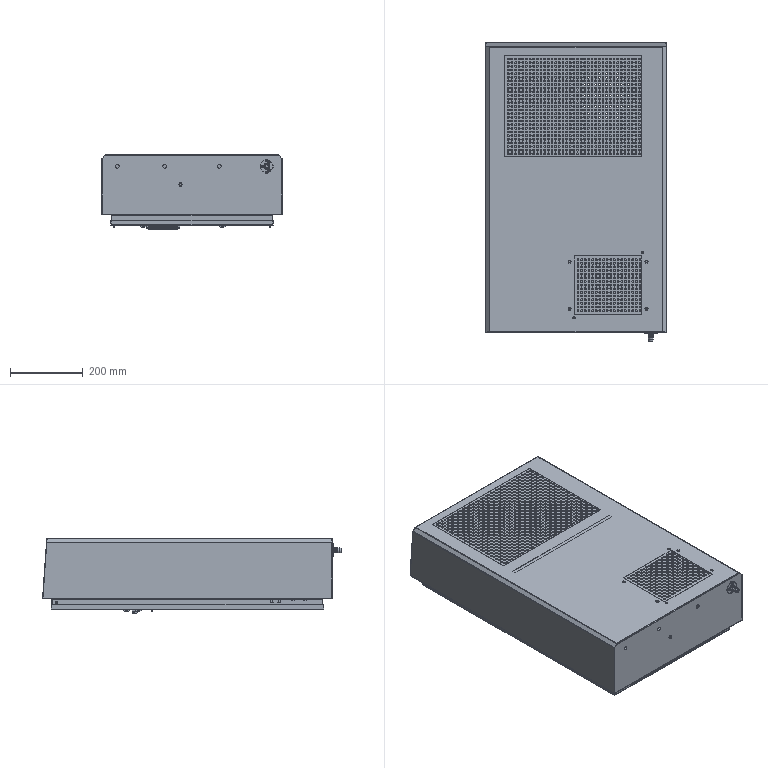Part | SolidWorks | features BaseBody 45 | 45 solids | 5675 faces | volume 1235769 mm3 | cylinder 3172 | plane 2018 | cone 353 | torus 84 | spline 48 | commonest cylinder face diameters 5 x2570 4 x142 4.5 x62 2 x38 4.2 x32 9 x30